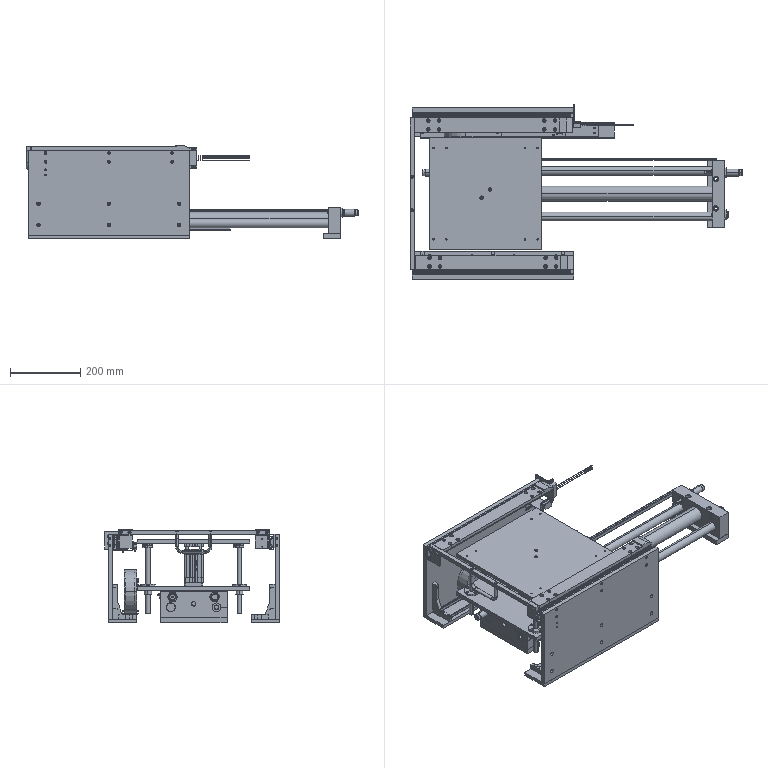Part | SolidWorks | features ReferencePattern 14, LocalLPattern 4, CompositeCurve 2 | 46 solids | 2859 faces | box 944.207 x 496.5 x 267 mm | volume 12174928 mm3 | cylinder 1403 | plane 1123 | cone 299 | spline 34 | commonest cylinder face diameters 4.5 x153 4.2 x132 5.5 x112 8 x111 1 x105 10 x92